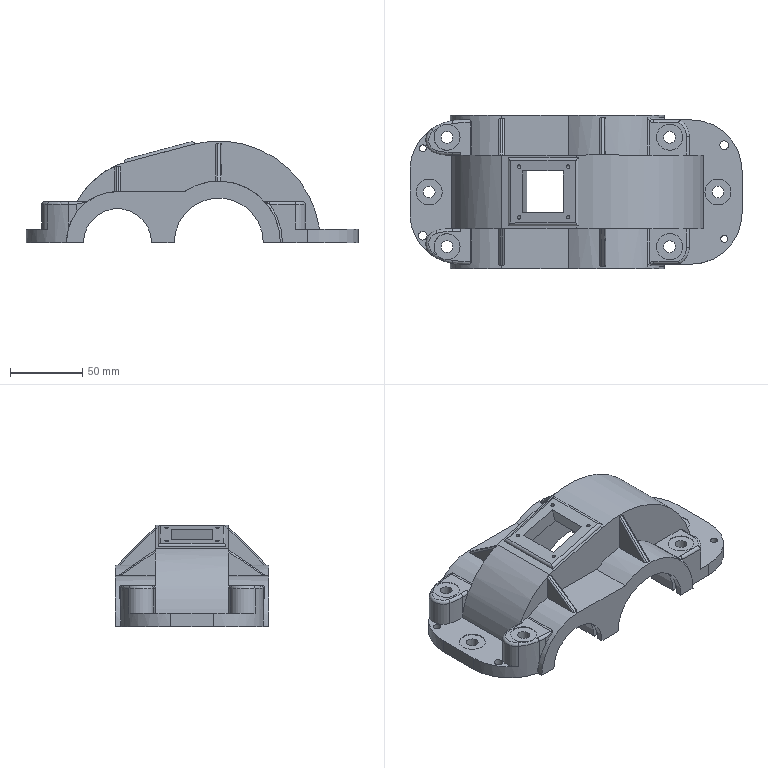Part | NX | features DATUM_CSYS 18, EXTRUDE 18, SKETCH 17, BLEND 13, EXTRACT_STRING 6, SYMBOLIC_THREAD 6, Instance Feature 4, Mirror Feature 4, RIB 4, ASSOCIATIVE_INTERSECTION 2, CHAMFER 2, DATUM_PLANE 2, EXTRACT_FACE 2, REPLACE_FACE 2 | 1 solid | 156 faces | box 229.56 x 106.4 x 70.29 mm | volume 339621 mm3 | cylinder 74 | plane 66 | torus 10 | spline 6 | commonest cylinder face diameters 4 x16 2 x8 8.2 x6 18 x6 70 x6 2.456 x4